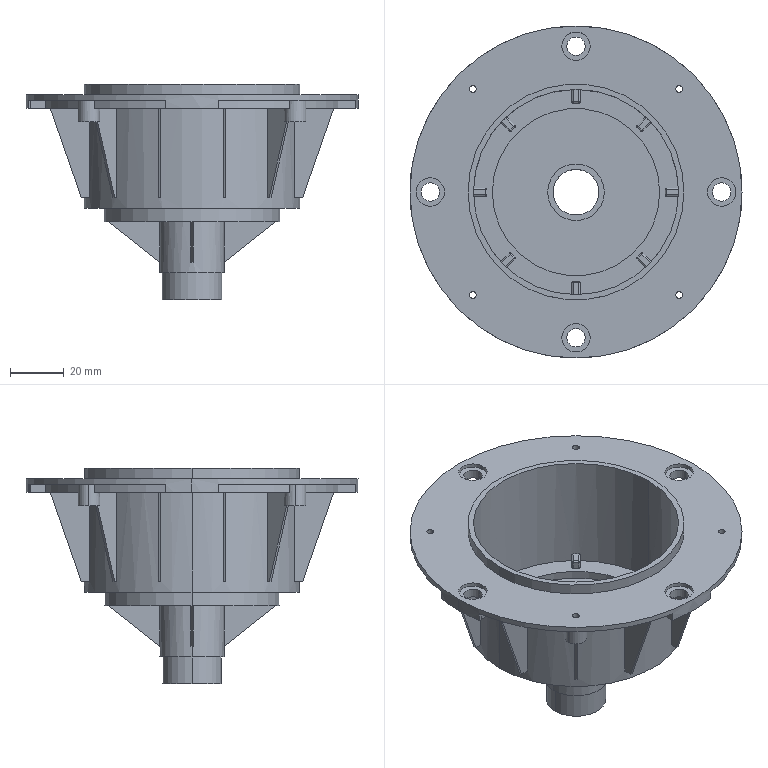Part | SolidWorks | features ICE 19, CirPattern 5, Rib 3, Extrusion 1, Fillet 1, MirrorPattern 1 | 1 solid | 287 faces | box 123 x 123 x 80 mm | volume 67941 mm3 | plane 142 | cylinder 128 | sphere 17 | commonest cylinder face diameters 1 x42 106 x16 8 x12 2.5 x8 6.8 x8 10.5 x8